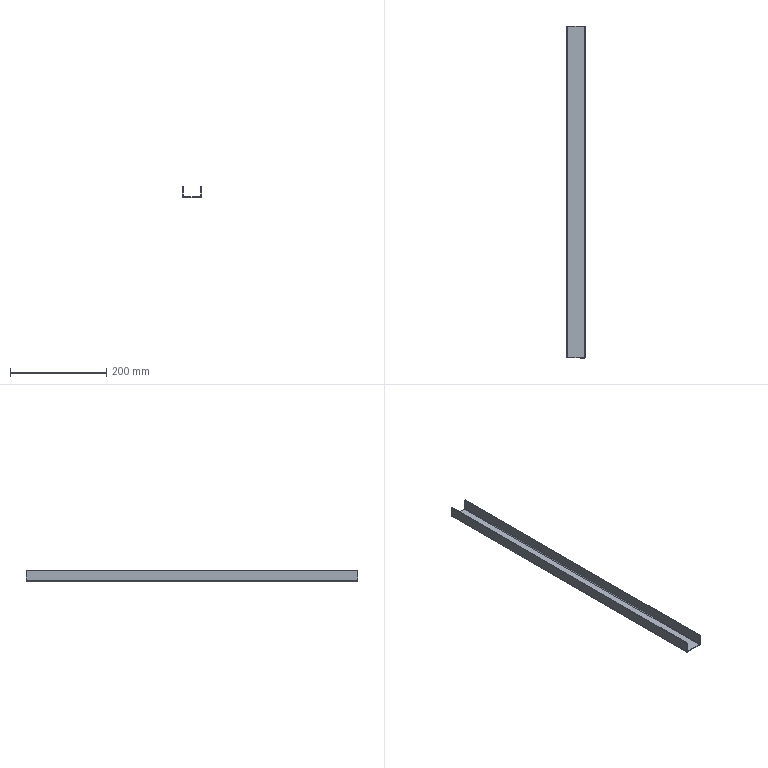Part | STEP file | Rear door reinforcing rib | 1 solid | 22 faces | box 40 x 691 x 23.5 mm | volume 85064 mm3 | plane 18 | cylinder 4 | commonest cylinder face diameters 3 x2 6 x2
STEP:
#1=CARTESIAN_POINT('',(0.,0.,0.));
#2=DIRECTION('',(0.,0.,1.));
#3=DIRECTION('',(1.,0.,0.));
#4=AXIS2_PLACEMENT_3D('',#1,#2,#3);
#5=CARTESIAN_POINT('',(-37.,0.,-1.5));
#6=VERTEX_POINT('',#5);
#7=CARTESIAN_POINT('',(-3.,0.,-1.5));
#8=VERTEX_POINT('',#7);
#9=CARTESIAN_POINT('',(0.,0.,-1.5));
#10=DIRECTION('',(1.,0.,0.));
#11=VECTOR('',#10,1.);
#12=LINE('',#9,#11);
#13=CARTESIAN_POINT('',(0.,0.,-1.5));
#14=DIRECTION('',(0.,0.,-1.));
#15=DIRECTION('',(-1.,0.,0.));
#16=AXIS2_PLACEMENT_3D('',#13,#14,#15);
#17=PLANE('',#16);
#18=CARTESIAN_POINT('',(0.,0.));
#19=DIRECTION('',(-1.,0.));
#20=VECTOR('',#19,1.);
#21=LINE('',#18,#20);
#22=(GEOMETRIC_REPRESENTATION_CONTEXT(2)PARAMETRIC_REPRESENTATION_CONTEXT()REPRESENTATION_CONTEXT('',''));
#23=DEFINITIONAL_REPRESENTATION('',(#21),#22);
#24=PCURVE('',#17,#23);
#25=CARTESIAN_POINT('',(0.,0.,-1.5));
#26=DIRECTION('',(0.,-1.,0.));
#27=DIRECTION('',(1.,0.,0.));
#28=AXIS2_PLACEMENT_3D('',#25,#26,#27);
#29=PLANE('',#28);
#30=CARTESIAN_POINT('',(0.,0.));
#31=DIRECTION('',(1.,0.));
#32=VECTOR('',#31,1.);
#33=LINE('',#30,#32);
#34=(GEOMETRIC_REPRESENTATION_CONTEXT(2)PARAMETRIC_REPRESENTATION_CONTEXT()REPRESENTATION_CONTEXT('',''));
#35=DEFINITIONAL_REPRESENTATION('',(#33),#34);
#36=PCURVE('',#29,#35);
#37=SURFACE_CURVE('',#12,(#24,#36),.PCURVE_S1.);
#38=EDGE_CURVE('',#6,#8,#37,.T.);
#39=ORIENTED_EDGE('',*,*,#38,.F.);
#40=CARTESIAN_POINT('',(-37.,691.,-1.5));
#41=VERTEX_POINT('',#40);
#42=CARTESIAN_POINT('',(-37.,0.,-1.5));
#43=DIRECTION('',(0.,1.,0.));
#44=VECTOR('',#43,1.);
#45=LINE('',#42,#44);
#46=CARTESIAN_POINT('',(37.,0.));
#47=DIRECTION('',(0.,1.));
#48=VECTOR('',#47,1.);
#49=LINE('',#46,#48);
#50=(GEOMETRIC_REPRESENTATION_CONTEXT(2)PARAMETRIC_REPRESENTATION_CONTEXT()REPRESENTATION_CONTEXT('',''));
#51=DEFINITIONAL_REPRESENTATION('',(#49),#50);
#52=PCURVE('',#17,#51);
#53=CARTESIAN_POINT('',(-37.,0.,1.5));
#54=DIRECTION('',(0.,-1.,0.));
#55=DIRECTION('',(-1.,0.,0.));
#56=AXIS2_PLACEMENT_3D('',#53,#54,#55);
#57=CYLINDRICAL_SURFACE('',#56,3.);
#58=CARTESIAN_POINT('',(1.571,0.));
#59=DIRECTION('',(0.,-1.));
#60=VECTOR('',#59,1.);
#61=LINE('',#58,#60);
#62=(GEOMETRIC_REPRESENTATION_CONTEXT(2)PARAMETRIC_REPRESENTATION_CONTEXT()REPRESENTATION_CONTEXT('',''));
#63=DEFINITIONAL_REPRESENTATION('',(#61),#62);
#64=PCURVE('',#57,#63);
#65=SURFACE_CURVE('',#45,(#52,#64),.PCURVE_S1.);
#66=EDGE_CURVE('',#6,#41,#65,.T.);
#67=ORIENTED_EDGE('',*,*,#66,.T.);
#68=CARTESIAN_POINT('',(-3.,691.,-1.5));
#69=VERTEX_POINT('',#68);
#70=CARTESIAN_POINT('',(0.,691.,-1.5));
#71=DIRECTION('',(-1.,0.,0.));
#72=VECTOR('',#71,1.);
#73=LINE('',#70,#72);
#74=CARTESIAN_POINT('',(0.,691.));
#75=DIRECTION('',(1.,0.));
#76=VECTOR('',#75,1.);
#77=LINE('',#74,#76);
#78=(GEOMETRIC_REPRESENTATION_CONTEXT(2)PARAMETRIC_REPRESENTATION_CONTEXT()REPRESENTATION_CONTEXT('',''));
#79=DEFINITIONAL_REPRESENTATION('',(#77),#78);
#80=PCURVE('',#17,#79);
#81=CARTESIAN_POINT('',(0.,691.,-1.5));
#82=DIRECTION('',(0.,1.,0.));
#83=DIRECTION('',(0.,0.,1.));
#84=AXIS2_PLACEMENT_3D('',#81,#82,#83);
#85=PLANE('',#84);
#86=CARTESIAN_POINT('',(0.,0.));
#87=DIRECTION('',(0.,-1.));
#88=VECTOR('',#87,1.);
#89=LINE('',#86,#88);
#90=(GEOMETRIC_REPRESENTATION_CONTEXT(2)PARAMETRIC_REPRESENTATION_CONTEXT()REPRESENTATION_CONTEXT('',''));
#91=DEFINITIONAL_REPRESENTATION('',(#89),#90);
#92=PCURVE('',#85,#91);
#93=SURFACE_CURVE('',#73,(#80,#92),.PCURVE_S1.);
#94=EDGE_CURVE('',#69,#41,#93,.T.);
#95=ORIENTED_EDGE('',*,*,#94,.F.);
#96=CARTESIAN_POINT('',(-3.,691.,-1.5));
#97=DIRECTION('',(0.,-1.,0.));
#98=VECTOR('',#97,1.);
#99=LINE('',#96,#98);
#100=CARTESIAN_POINT('',(3.,691.));
#101=DIRECTION('',(0.,-1.));
#102=VECTOR('',#101,1.);
#103=LINE('',#100,#102);
#104=(GEOMETRIC_REPRESENTATION_CONTEXT(2)PARAMETRIC_REPRESENTATION_CONTEXT()REPRESENTATION_CONTEXT('',''));
#105=DEFINITIONAL_REPRESENTATION('',(#103),#104);
#106=PCURVE('',#17,#105);
#107=CARTESIAN_POINT('',(-3.,691.,1.5));
#108=DIRECTION('',(0.,1.,0.));
#109=DIRECTION('',(1.,0.,0.));
#110=AXIS2_PLACEMENT_3D('',#107,#108,#109);
#111=CYLINDRICAL_SURFACE('',#110,3.);
#112=CARTESIAN_POINT('',(1.571,0.));
#113=DIRECTION('',(0.,-1.));
#114=VECTOR('',#113,1.);
#115=LINE('',#112,#114);
#116=(GEOMETRIC_REPRESENTATION_CONTEXT(2)PARAMETRIC_REPRESENTATION_CONTEXT()REPRESENTATION_CONTEXT('',''));
#117=DEFINITIONAL_REPRESENTATION('',(#115),#116);
#118=PCURVE('',#111,#117);
#119=SURFACE_CURVE('',#99,(#106,#118),.PCURVE_S1.);
#120=EDGE_CURVE('',#69,#8,#119,.T.);
#121=ORIENTED_EDGE('',*,*,#120,.T.);
#122=EDGE_LOOP('',(#39,#67,#95,#121));
#123=FACE_BOUND('',#122,.T.);
#124=ADVANCED_FACE('',(#123),#17,.T.);
#125=CARTESIAN_POINT('',(-37.,0.,0.));
#126=VERTEX_POINT('',#125);
#127=CARTESIAN_POINT('',(-37.,691.,0.));
#128=VERTEX_POINT('',#127);
#129=CARTESIAN_POINT('',(-37.,0.,0.));
#130=DIRECTION('',(0.,1.,0.));
#131=VECTOR('',#130,1.);
#132=LINE('',#129,#131);
#133=CARTESIAN_POINT('',(0.,0.,0.));
#134=DIRECTION('',(0.,0.,-1.));
#135=DIRECTION('',(-1.,0.,0.));
#136=AXIS2_PLACEMENT_3D('',#133,#134,#135);
#137=PLANE('',#136);
#138=CARTESIAN_POINT('',(37.,0.));
#139=DIRECTION('',(0.,1.));
#140=VECTOR('',#139,1.);
#141=LINE('',#138,#140);
#142=(GEOMETRIC_REPRESENTATION_CONTEXT(2)PARAMETRIC_REPRESENTATION_CONTEXT()REPRESENTATION_CONTEXT('',''));
#143=DEFINITIONAL_REPRESENTATION('',(#141),#142);
#144=PCURVE('',#137,#143);
#145=CARTESIAN_POINT('',(-37.,0.,1.5));
#146=DIRECTION('',(0.,-1.,0.));
#147=DIRECTION('',(-1.,0.,0.));
#148=AXIS2_PLACEMENT_3D('',#145,#146,#147);
#149=CYLINDRICAL_SURFACE('',#148,1.5);
#150=CARTESIAN_POINT('',(1.571,0.));
#151=DIRECTION('',(0.,-1.));
#152=VECTOR('',#151,1.);
#153=LINE('',#150,#152);
#154=(GEOMETRIC_REPRESENTATION_CONTEXT(2)PARAMETRIC_REPRESENTATION_CONTEXT()REPRESENTATION_CONTEXT('',''));
#155=DEFINITIONAL_REPRESENTATION('',(#153),#154);
#156=PCURVE('',#149,#155);
#157=SURFACE_CURVE('',#132,(#144,#156),.PCURVE_S1.);
#158=EDGE_CURVE('',#126,#128,#157,.T.);
#159=ORIENTED_EDGE('',*,*,#158,.F.);
#160=CARTESIAN_POINT('',(-3.,0.,0.));
#161=VERTEX_POINT('',#160);
#162=CARTESIAN_POINT('',(0.,0.,0.));
#163=DIRECTION('',(1.,0.,0.));
#164=VECTOR('',#163,1.);
#165=LINE('',#162,#164);
#166=CARTESIAN_POINT('',(0.,0.));
#167=DIRECTION('',(-1.,0.));
#168=VECTOR('',#167,1.);
#169=LINE('',#166,#168);
#170=(GEOMETRIC_REPRESENTATION_CONTEXT(2)PARAMETRIC_REPRESENTATION_CONTEXT()REPRESENTATION_CONTEXT('',''));
#171=DEFINITIONAL_REPRESENTATION('',(#169),#170);
#172=PCURVE('',#137,#171);
#173=CARTESIAN_POINT('',(0.,1.5));
#174=DIRECTION('',(1.,0.));
#175=VECTOR('',#174,1.);
#176=LINE('',#173,#175);
#177=(GEOMETRIC_REPRESENTATION_CONTEXT(2)PARAMETRIC_REPRESENTATION_CONTEXT()REPRESENTATION_CONTEXT('',''));
#178=DEFINITIONAL_REPRESENTATION('',(#176),#177);
#179=PCURVE('',#29,#178);
#180=SURFACE_CURVE('',#165,(#172,#179),.PCURVE_S1.);
#181=EDGE_CURVE('',#126,#161,#180,.T.);
#182=ORIENTED_EDGE('',*,*,#181,.T.);
#183=CARTESIAN_POINT('',(-3.,691.,0.));
#184=VERTEX_POINT('',#183);
#185=CARTESIAN_POINT('',(-3.,691.,0.));
#186=DIRECTION('',(0.,-1.,0.));
#187=VECTOR('',#186,1.);
#188=LINE('',#185,#187);
#189=CARTESIAN_POINT('',(3.,691.));
#190=DIRECTION('',(0.,-1.));
#191=VECTOR('',#190,1.);
#192=LINE('',#189,#191);
#193=(GEOMETRIC_REPRESENTATION_CONTEXT(2)PARAMETRIC_REPRESENTATION_CONTEXT()REPRESENTATION_CONTEXT('',''));
#194=DEFINITIONAL_REPRESENTATION('',(#192),#193);
#195=PCURVE('',#137,#194);
#196=CARTESIAN_POINT('',(-3.,691.,1.5));
#197=DIRECTION('',(0.,1.,0.));
#198=DIRECTION('',(1.,0.,0.));
#199=AXIS2_PLACEMENT_3D('',#196,#197,#198);
#200=CYLINDRICAL_SURFACE('',#199,1.5);
#201=CARTESIAN_POINT('',(1.571,0.));
#202=DIRECTION('',(0.,-1.));
#203=VECTOR('',#202,1.);
#204=LINE('',#201,#203);
#205=(GEOMETRIC_REPRESENTATION_CONTEXT(2)PARAMETRIC_REPRESENTATION_CONTEXT()REPRESENTATION_CONTEXT('',''));
#206=DEFINITIONAL_REPRESENTATION('',(#204),#205);
#207=PCURVE('',#200,#206);
#208=SURFACE_CURVE('',#188,(#195,#207),.PCURVE_S1.);
#209=EDGE_CURVE('',#184,#161,#208,.T.);
#210=ORIENTED_EDGE('',*,*,#209,.F.);
#211=CARTESIAN_POINT('',(0.,691.,0.));
#212=DIRECTION('',(-1.,0.,0.));
#213=VECTOR('',#212,1.);
#214=LINE('',#211,#213);
#215=CARTESIAN_POINT('',(0.,691.));
#216=DIRECTION('',(1.,0.));
#217=VECTOR('',#216,1.);
#218=LINE('',#215,#217);
#219=(GEOMETRIC_REPRESENTATION_CONTEXT(2)PARAMETRIC_REPRESENTATION_CONTEXT()REPRESENTATION_CONTEXT('',''));
#220=DEFINITIONAL_REPRESENTATION('',(#218),#219);
#221=PCURVE('',#137,#220);
#222=CARTESIAN_POINT('',(1.5,0.));
#223=DIRECTION('',(0.,-1.));
#224=VECTOR('',#223,1.);
#225=LINE('',#222,#224);
#226=(GEOMETRIC_REPRESENTATION_CONTEXT(2)PARAMETRIC_REPRESENTATION_CONTEXT()REPRESENTATION_CONTEXT('',''));
#227=DEFINITIONAL_REPRESENTATION('',(#225),#226);
#228=PCURVE('',#85,#227);
#229=SURFACE_CURVE('',#214,(#221,#228),.PCURVE_S1.);
#230=EDGE_CURVE('',#184,#128,#229,.T.);
#231=ORIENTED_EDGE('',*,*,#230,.T.);
#232=EDGE_LOOP('',(#159,#182,#210,#231));
#233=FACE_BOUND('',#232,.T.);
#234=ADVANCED_FACE('',(#233),#137,.F.);
#235=ORIENTED_EDGE('',*,*,#181,.F.);
#236=CARTESIAN_POINT('',(-37.,0.,0.));
#237=DIRECTION('',(0.,0.,-1.));
#238=VECTOR('',#237,1.);
#239=LINE('',#236,#238);
#240=CARTESIAN_POINT('',(-37.,1.5));
#241=DIRECTION('',(0.,-1.));
#242=VECTOR('',#241,1.);
#243=LINE('',#240,#242);
#244=(GEOMETRIC_REPRESENTATION_CONTEXT(2)PARAMETRIC_REPRESENTATION_CONTEXT()REPRESENTATION_CONTEXT('',''));
#245=DEFINITIONAL_REPRESENTATION('',(#243),#244);
#246=PCURVE('',#29,#245);
#247=CARTESIAN_POINT('',(-37.,0.,1.5));
#248=DIRECTION('',(0.,1.,0.));
#249=DIRECTION('',(0.,0.,1.));
#250=AXIS2_PLACEMENT_3D('',#247,#248,#249);
#251=PLANE('',#250);
#252=CARTESIAN_POINT('',(-1.5,0.));
#253=DIRECTION('',(-1.,0.));
#254=VECTOR('',#253,1.);
#255=LINE('',#252,#254);
#256=(GEOMETRIC_REPRESENTATION_CONTEXT(2)PARAMETRIC_REPRESENTATION_CONTEXT()REPRESENTATION_CONTEXT('',''));
#257=DEFINITIONAL_REPRESENTATION('',(#255),#256);
#258=PCURVE('',#251,#257);
#259=SURFACE_CURVE('',#239,(#246,#258),.PCURVE_S1.);
#260=EDGE_CURVE('',#126,#6,#259,.T.);
#261=ORIENTED_EDGE('',*,*,#260,.T.);
#262=ORIENTED_EDGE('',*,*,#38,.T.);
#263=CARTESIAN_POINT('',(-3.,0.,0.));
#264=DIRECTION('',(0.,0.,-1.));
#265=VECTOR('',#264,1.);
#266=LINE('',#263,#265);
#267=CARTESIAN_POINT('',(-3.,1.5));
#268=DIRECTION('',(0.,-1.));
#269=VECTOR('',#268,1.);
#270=LINE('',#267,#269);
#271=(GEOMETRIC_REPRESENTATION_CONTEXT(2)PARAMETRIC_REPRESENTATION_CONTEXT()REPRESENTATION_CONTEXT('',''));
#272=DEFINITIONAL_REPRESENTATION('',(#270),#271);
#273=PCURVE('',#29,#272);
#274=CARTESIAN_POINT('',(-3.,0.,1.5));
#275=DIRECTION('',(0.,-1.,0.));
#276=DIRECTION('',(1.,0.,0.));
#277=AXIS2_PLACEMENT_3D('',#274,#275,#276);
#278=PLANE('',#277);
#279=CARTESIAN_POINT('',(0.,-1.5));
#280=DIRECTION('',(0.,-1.));
#281=VECTOR('',#280,1.);
#282=LINE('',#279,#281);
#283=(GEOMETRIC_REPRESENTATION_CONTEXT(2)PARAMETRIC_REPRESENTATION_CONTEXT()REPRESENTATION_CONTEXT('',''));
#284=DEFINITIONAL_REPRESENTATION('',(#282),#283);
#285=PCURVE('',#278,#284);
#286=SURFACE_CURVE('',#266,(#273,#285),.PCURVE_S1.);
#287=EDGE_CURVE('',#161,#8,#286,.T.);
#288=ORIENTED_EDGE('',*,*,#287,.F.);
#289=EDGE_LOOP('',(#235,#261,#262,#288));
#290=FACE_BOUND('',#289,.T.);
#291=ADVANCED_FACE('',(#290),#29,.T.);
#292=CARTESIAN_POINT('',(-37.,691.,0.));
#293=DIRECTION('',(0.,0.,-1.));
#294=VECTOR('',#293,1.);
#295=LINE('',#292,#294);
#296=CARTESIAN_POINT('',(1.5,-37.));
#297=DIRECTION('',(-1.,0.));
#298=VECTOR('',#297,1.);
#299=LINE('',#296,#298);
#300=(GEOMETRIC_REPRESENTATION_CONTEXT(2)PARAMETRIC_REPRESENTATION_CONTEXT()REPRESENTATION_CONTEXT('',''));
#301=DEFINITIONAL_REPRESENTATION('',(#299),#300);
#302=PCURVE('',#85,#301);
#303=CARTESIAN_POINT('',(-37.,691.,1.5));
#304=DIRECTION('',(0.,1.,0.));
#305=DIRECTION('',(0.,0.,1.));
#306=AXIS2_PLACEMENT_3D('',#303,#304,#305);
#307=PLANE('',#306);
#308=CARTESIAN_POINT('',(-1.5,0.));
#309=DIRECTION('',(-1.,0.));
#310=VECTOR('',#309,1.);
#311=LINE('',#308,#310);
#312=(GEOMETRIC_REPRESENTATION_CONTEXT(2)PARAMETRIC_REPRESENTATION_CONTEXT()REPRESENTATION_CONTEXT('',''));
#313=DEFINITIONAL_REPRESENTATION('',(#311),#312);
#314=PCURVE('',#307,#313);
#315=SURFACE_CURVE('',#295,(#302,#314),.PCURVE_S1.);
#316=EDGE_CURVE('',#128,#41,#315,.T.);
#317=ORIENTED_EDGE('',*,*,#316,.F.);
#318=ORIENTED_EDGE('',*,*,#230,.F.);
#319=CARTESIAN_POINT('',(-3.,691.,0.));
#320=DIRECTION('',(0.,0.,-1.));
#321=VECTOR('',#320,1.);
#322=LINE('',#319,#321);
#323=CARTESIAN_POINT('',(1.5,-3.));
#324=DIRECTION('',(-1.,0.));
#325=VECTOR('',#324,1.);
#326=LINE('',#323,#325);
#327=(GEOMETRIC_REPRESENTATION_CONTEXT(2)PARAMETRIC_REPRESENTATION_CONTEXT()REPRESENTATION_CONTEXT('',''));
#328=DEFINITIONAL_REPRESENTATION('',(#326),#327);
#329=PCURVE('',#85,#328);
#330=CARTESIAN_POINT('',(-3.,691.,1.5));
#331=DIRECTION('',(0.,-1.,0.));
#332=DIRECTION('',(1.,0.,0.));
#333=AXIS2_PLACEMENT_3D('',#330,#331,#332);
#334=PLANE('',#333);
#335=CARTESIAN_POINT('',(0.,-1.5));
#336=DIRECTION('',(0.,-1.));
#337=VECTOR('',#336,1.);
#338=LINE('',#335,#337);
#339=(GEOMETRIC_REPRESENTATION_CONTEXT(2)PARAMETRIC_REPRESENTATION_CONTEXT()REPRESENTATION_CONTEXT('',''));
#340=DEFINITIONAL_REPRESENTATION('',(#338),#339);
#341=PCURVE('',#334,#340);
#342=SURFACE_CURVE('',#322,(#329,#341),.PCURVE_S1.);
#343=EDGE_CURVE('',#184,#69,#342,.T.);
#344=ORIENTED_EDGE('',*,*,#343,.T.);
#345=ORIENTED_EDGE('',*,*,#94,.T.);
#346=EDGE_LOOP('',(#317,#318,#344,#345));
#347=FACE_BOUND('',#346,.T.);
#348=ADVANCED_FACE('',(#347),#85,.T.);
#349=CARTESIAN_POINT('',(-1.5,0.,1.5));
#350=VERTEX_POINT('',#349);
#351=CARTESIAN_POINT('',(0.,0.,1.5));
#352=VERTEX_POINT('',#351);
#353=CARTESIAN_POINT('',(0.,0.,1.5));
#354=DIRECTION('',(1.,0.,0.));
#355=VECTOR('',#354,1.);
#356=LINE('',#353,#355);
#357=CARTESIAN_POINT('',(3.,0.));
#358=DIRECTION('',(1.,0.));
#359=VECTOR('',#358,1.);
#360=LINE('',#357,#359);
#361=(GEOMETRIC_REPRESENTATION_CONTEXT(2)PARAMETRIC_REPRESENTATION_CONTEXT()REPRESENTATION_CONTEXT('',''));
#362=DEFINITIONAL_REPRESENTATION('',(#360),#361);
#363=PCURVE('',#278,#362);
#364=CARTESIAN_POINT('',(0.,0.,0.));
#365=DIRECTION('',(0.,1.,0.));
#366=DIRECTION('',(-1.,0.,0.));
#367=AXIS2_PLACEMENT_3D('',#364,#365,#366);
#368=PLANE('',#367);
#369=CARTESIAN_POINT('',(0.,1.5));
#370=DIRECTION('',(-1.,0.));
#371=VECTOR('',#370,1.);
#372=LINE('',#369,#371);
#373=(GEOMETRIC_REPRESENTATION_CONTEXT(2)PARAMETRIC_REPRESENTATION_CONTEXT()REPRESENTATION_CONTEXT('',''));
#374=DEFINITIONAL_REPRESENTATION('',(#372),#373);
#375=PCURVE('',#368,#374);
#376=SURFACE_CURVE('',#356,(#363,#375),.PCURVE_S1.);
#377=EDGE_CURVE('',#350,#352,#376,.T.);
#378=ORIENTED_EDGE('',*,*,#377,.F.);
#379=CARTESIAN_POINT('',(-3.,0.,1.5));
#380=DIRECTION('',(0.,-1.,0.));
#381=DIRECTION('',(-1.,0.,0.));
#382=AXIS2_PLACEMENT_3D('',#379,#380,#381);
#383=CIRCLE('',#382,1.5);
#384=CARTESIAN_POINT('',(0.,0.));
#385=DIRECTION('',(-1.,0.));
#386=AXIS2_PLACEMENT_2D('',#384,#385);
#387=CIRCLE('',#386,1.5);
#388=(GEOMETRIC_REPRESENTATION_CONTEXT(2)PARAMETRIC_REPRESENTATION_CONTEXT()REPRESENTATION_CONTEXT('',''));
#389=DEFINITIONAL_REPRESENTATION('',(#387),#388);
#390=PCURVE('',#278,#389);
#391=CARTESIAN_POINT('',(3.142,-691.));
#392=DIRECTION('',(-1.,0.));
#393=VECTOR('',#392,1.);
#394=LINE('',#391,#393);
#395=(GEOMETRIC_REPRESENTATION_CONTEXT(2)PARAMETRIC_REPRESENTATION_CONTEXT()REPRESENTATION_CONTEXT('',''));
#396=DEFINITIONAL_REPRESENTATION('',(#394),#395);
#397=PCURVE('',#200,#396);
#398=SURFACE_CURVE('',#383,(#390,#397),.PCURVE_S1.);
#399=EDGE_CURVE('',#161,#350,#398,.T.);
#400=ORIENTED_EDGE('',*,*,#399,.F.);
#401=ORIENTED_EDGE('',*,*,#287,.T.);
#402=CARTESIAN_POINT('',(-3.,0.,1.5));
#403=DIRECTION('',(0.,-1.,0.));
#404=DIRECTION('',(-1.,0.,0.));
#405=AXIS2_PLACEMENT_3D('',#402,#403,#404);
#406=CIRCLE('',#405,3.);
#407=CARTESIAN_POINT('',(0.,0.));
#408=DIRECTION('',(-1.,0.));
#409=AXIS2_PLACEMENT_2D('',#407,#408);
#410=CIRCLE('',#409,3.);
#411=(GEOMETRIC_REPRESENTATION_CONTEXT(2)PARAMETRIC_REPRESENTATION_CONTEXT()REPRESENTATION_CONTEXT('',''));
#412=DEFINITIONAL_REPRESENTATION('',(#410),#411);
#413=PCURVE('',#278,#412);
#414=CARTESIAN_POINT('',(3.142,-691.));
#415=DIRECTION('',(-1.,0.));
#416=VECTOR('',#415,1.);
#417=LINE('',#414,#416);
#418=(GEOMETRIC_REPRESENTATION_CONTEXT(2)PARAMETRIC_REPRESENTATION_CONTEXT()REPRESENTATION_CONTEXT('',''));
#419=DEFINITIONAL_REPRESENTATION('',(#417),#418);
#420=PCURVE('',#111,#419);
#421=SURFACE_CURVE('',#406,(#413,#420),.PCURVE_S1.);
#422=EDGE_CURVE('',#8,#352,#421,.T.);
#423=ORIENTED_EDGE('',*,*,#422,.T.);
#424=EDGE_LOOP('',(#378,#400,#401,#423));
#425=FACE_BOUND('',#424,.T.);
#426=ADVANCED_FACE('',(#425),#278,.T.);
#427=CARTESIAN_POINT('',(-1.5,691.,1.5));
#428=VERTEX_POINT('',#427);
#429=CARTESIAN_POINT('',(-3.,691.,1.5));
#430=DIRECTION('',(0.,1.,0.));
#431=DIRECTION('',(-1.,0.,0.));
#432=AXIS2_PLACEMENT_3D('',#429,#430,#431);
#433=CIRCLE('',#432,1.5);
#434=CARTESIAN_POINT('',(-1.5,0.));
#435=CARTESIAN_POINT('',(-1.5,2.598));
#436=CARTESIAN_POINT('',(0.75,1.299));
#437=CARTESIAN_POINT('',(3.,0.));
#438=CARTESIAN_POINT('',(0.75,-1.299));
#439=CARTESIAN_POINT('',(-1.5,-2.598));
#440=CARTESIAN_POINT('',(-1.5,0.));
#441=(BOUNDED_CURVE()B_SPLINE_CURVE(2,(#434,#435,#436,#437,#438,#439,#440),.UNSPECIFIED.,.T.,.F.)B_SPLINE_CURVE_WITH_KNOTS((1,2,2,2,2,1),(-2.094,0.,2.094,4.189,6.283,8.378),.UNSPECIFIED.)CURVE()GEOMETRIC_REPRESENTATION_ITEM()RATIONAL_B_SPLINE_CURVE((1.,0.5,1.,0.5,1.,0.5,1.))REPRESENTATION_ITEM(''));
#442=(GEOMETRIC_REPRESENTATION_CONTEXT(2)PARAMETRIC_REPRESENTATION_CONTEXT()REPRESENTATION_CONTEXT('',''));
#443=DEFINITIONAL_REPRESENTATION('',(#441),#442);
#444=PCURVE('',#334,#443);
#445=CARTESIAN_POINT('',(-3.142,0.));
#446=DIRECTION('',(1.,0.));
#447=VECTOR('',#446,1.);
#448=LINE('',#445,#447);
#449=(GEOMETRIC_REPRESENTATION_CONTEXT(2)PARAMETRIC_REPRESENTATION_CONTEXT()REPRESENTATION_CONTEXT('',''));
#450=DEFINITIONAL_REPRESENTATION('',(#448),#449);
#451=PCURVE('',#200,#450);
#452=SURFACE_CURVE('',#433,(#444,#451),.PCURVE_S1.);
#453=EDGE_CURVE('',#428,#184,#452,.T.);
#454=ORIENTED_EDGE('',*,*,#453,.F.);
#455=CARTESIAN_POINT('',(0.,691.,1.5));
#456=VERTEX_POINT('',#455);
#457=CARTESIAN_POINT('',(-1.5,691.,1.5));
#458=DIRECTION('',(1.,0.,0.));
#459=VECTOR('',#458,1.);
#460=LINE('',#457,#459);
#461=CARTESIAN_POINT('',(1.5,0.));
#462=DIRECTION('',(1.,0.));
#463=VECTOR('',#462,1.);
#464=LINE('',#461,#463);
#465=(GEOMETRIC_REPRESENTATION_CONTEXT(2)PARAMETRIC_REPRESENTATION_CONTEXT()REPRESENTATION_CONTEXT('',''));
#466=DEFINITIONAL_REPRESENTATION('',(#464),#465);
#467=PCURVE('',#334,#466);
#468=CARTESIAN_POINT('',(0.,691.,22.));
#469=DIRECTION('',(0.,-1.,0.));
#470=DIRECTION('',(1.,0.,0.));
#471=AXIS2_PLACEMENT_3D('',#468,#469,#470);
#472=PLANE('',#471);
#473=CARTESIAN_POINT('',(-1.5,-20.5));
#474=DIRECTION('',(1.,0.));
#475=VECTOR('',#474,1.);
#476=LINE('',#473,#475);
#477=(GEOMETRIC_REPRESENTATION_CONTEXT(2)PARAMETRIC_REPRESENTATION_CONTEXT()REPRESENTATION_CONTEXT('',''));
#478=DEFINITIONAL_REPRESENTATION('',(#476),#477);
#479=PCURVE('',#472,#478);
#480=SURFACE_CURVE('',#460,(#467,#479),.PCURVE_S1.);
#481=EDGE_CURVE('',#428,#456,#480,.T.);
#482=ORIENTED_EDGE('',*,*,#481,.T.);
#483=CARTESIAN_POINT('',(-3.,691.,1.5));
#484=DIRECTION('',(0.,1.,0.));
#485=DIRECTION('',(-1.,0.,0.));
#486=AXIS2_PLACEMENT_3D('',#483,#484,#485);
#487=CIRCLE('',#486,3.);
#488=CARTESIAN_POINT('',(-3.,0.));
#489=CARTESIAN_POINT('',(-3.,5.196));
#490=CARTESIAN_POINT('',(1.5,2.598));
#491=CARTESIAN_POINT('',(6.,0.));
#492=CARTESIAN_POINT('',(1.5,-2.598));
#493=CARTESIAN_POINT('',(-3.,-5.196));
#494=CARTESIAN_POINT('',(-3.,0.));
#495=(BOUNDED_CURVE()B_SPLINE_CURVE(2,(#488,#489,#490,#491,#492,#493,#494),.UNSPECIFIED.,.T.,.F.)B_SPLINE_CURVE_WITH_KNOTS((1,2,2,2,2,1),(-2.094,0.,2.094,4.189,6.283,8.378),.UNSPECIFIED.)CURVE()GEOMETRIC_REPRESENTATION_ITEM()RATIONAL_B_SPLINE_CURVE((1.,0.5,1.,0.5,1.,0.5,1.))REPRESENTATION_ITEM(''));
#496=(GEOMETRIC_REPRESENTATION_CONTEXT(2)PARAMETRIC_REPRESENTATION_CONTEXT()REPRESENTATION_CONTEXT('',''));
#497=DEFINITIONAL_REPRESENTATION('',(#495),#496);
#498=PCURVE('',#334,#497);
#499=CARTESIAN_POINT('',(-3.142,0.));
#500=DIRECTION('',(1.,0.));
#501=VECTOR('',#500,1.);
#502=LINE('',#499,#501);
#503=(GEOMETRIC_REPRESENTATION_CONTEXT(2)PARAMETRIC_REPRESENTATION_CONTEXT()REPRESENTATION_CONTEXT('',''));
#504=DEFINITIONAL_REPRESENTATION('',(#502),#503);
#505=PCURVE('',#111,#504);
#506=SURFACE_CURVE('',#487,(#498,#505),.PCURVE_S1.);
#507=EDGE_CURVE('',#456,#69,#506,.T.);
#508=ORIENTED_EDGE('',*,*,#507,.T.);
#509=ORIENTED_EDGE('',*,*,#343,.F.);
#510=EDGE_LOOP('',(#454,#482,#508,#509));
#511=FACE_BOUND('',#510,.T.);
#512=ADVANCED_FACE('',(#511),#334,.F.);
#513=ORIENTED_EDGE('',*,*,#120,.F.);
#514=ORIENTED_EDGE('',*,*,#507,.F.);
#515=CARTESIAN_POINT('',(0.,0.,1.5));
#516=DIRECTION('',(0.,-1.,0.));
#517=VECTOR('',#516,1.);
#518=LINE('',#515,#517);
#519=CARTESIAN_POINT('',(0.,-691.));
#520=DIRECTION('',(0.,-1.));
#521=VECTOR('',#520,1.);
#522=LINE('',#519,#521);
#523=(GEOMETRIC_REPRESENTATION_CONTEXT(2)PARAMETRIC_REPRESENTATION_CONTEXT()REPRESENTATION_CONTEXT('',''));
#524=DEFINITIONAL_REPRESENTATION('',(#522),#523);
#525=PCURVE('',#111,#524);
#526=CARTESIAN_POINT('',(0.,0.,0.));
#527=DIRECTION('',(-1.,0.,0.));
#528=DIRECTION('',(0.,0.,1.));
#529=AXIS2_PLACEMENT_3D('',#526,#527,#528);
#530=PLANE('',#529);
#531=CARTESIAN_POINT('',(1.5,0.));
#532=DIRECTION('',(0.,-1.));
#533=VECTOR('',#532,1.);
#534=LINE('',#531,#533);
#535=(GEOMETRIC_REPRESENTATION_CONTEXT(2)PARAMETRIC_REPRESENTATION_CONTEXT()REPRESENTATION_CONTEXT('',''));
#536=DEFINITIONAL_REPRESENTATION('',(#534),#535);
#537=PCURVE('',#530,#536);
#538=SURFACE_CURVE('',#518,(#525,#537),.PCURVE_S1.);
#539=EDGE_CURVE('',#456,#352,#538,.T.);
#540=ORIENTED_EDGE('',*,*,#539,.T.);
#541=ORIENTED_EDGE('',*,*,#422,.F.);
#542=EDGE_LOOP('',(#513,#514,#540,#541));
#543=FACE_BOUND('',#542,.T.);
#544=ADVANCED_FACE('',(#543),#111,.T.);
#545=ORIENTED_EDGE('',*,*,#453,.F.);
#546=CARTESIAN_POINT('',(-1.5,0.,1.5));
#547=DIRECTION('',(0.,1.,0.));
#548=VECTOR('',#547,1.);
#549=LINE('',#546,#548);
#550=CARTESIAN_POINT('',(0.,-691.));
#551=DIRECTION('',(0.,1.));
#552=VECTOR('',#551,1.);
#553=LINE('',#550,#552);
#554=(GEOMETRIC_REPRESENTATION_CONTEXT(2)PARAMETRIC_REPRESENTATION_CONTEXT()REPRESENTATION_CONTEXT('',''));
#555=DEFINITIONAL_REPRESENTATION('',(#553),#554);
#556=PCURVE('',#200,#555);
#557=CARTESIAN_POINT('',(-1.5,0.,0.));
#558=DIRECTION('',(-1.,0.,0.));
#559=DIRECTION('',(0.,0.,1.));
#560=AXIS2_PLACEMENT_3D('',#557,#558,#559);
#561=PLANE('',#560);
#562=CARTESIAN_POINT('',(1.5,0.));
#563=DIRECTION('',(0.,1.));
#564=VECTOR('',#563,1.);
#565=LINE('',#562,#564);
#566=(GEOMETRIC_REPRESENTATION_CONTEXT(2)PARAMETRIC_REPRESENTATION_CONTEXT()REPRESENTATION_CONTEXT('',''));
#567=DEFINITIONAL_REPRESENTATION('',(#565),#566);
#568=PCURVE('',#561,#567);
#569=SURFACE_CURVE('',#549,(#556,#568),.PCURVE_S1.);
#570=EDGE_CURVE('',#350,#428,#569,.T.);
#571=ORIENTED_EDGE('',*,*,#570,.F.);
#572=ORIENTED_EDGE('',*,*,#399,.F.);
#573=ORIENTED_EDGE('',*,*,#209,.F.);
#574=EDGE_LOOP('',(#545,#571,#572,#573));
#575=FACE_BOUND('',#574,.F.);
#576=ADVANCED_FACE('',(#575),#200,.F.);
#577=ORIENTED_EDGE('',*,*,#377,.T.);
#578=CARTESIAN_POINT('',(0.,0.,22.));
#579=VERTEX_POINT('',#578);
#580=CARTESIAN_POINT('',(0.,0.,0.));
#581=DIRECTION('',(0.,0.,-1.));
#582=VECTOR('',#581,1.);
#583=LINE('',#580,#582);
#584=CARTESIAN_POINT('',(0.,0.));
#585=DIRECTION('',(0.,-1.));
#586=VECTOR('',#585,1.);
#587=LINE('',#584,#586);
#588=(GEOMETRIC_REPRESENTATION_CONTEXT(2)PARAMETRIC_REPRESENTATION_CONTEXT()REPRESENTATION_CONTEXT('',''));
#589=DEFINITIONAL_REPRESENTATION('',(#587),#588);
#590=PCURVE('',#368,#589);
#591=CARTESIAN_POINT('',(0.,0.));
#592=DIRECTION('',(-1.,0.));
#593=VECTOR('',#592,1.);
#594=LINE('',#591,#593);
#595=(GEOMETRIC_REPRESENTATION_CONTEXT(2)PARAMETRIC_REPRESENTATION_CONTEXT()REPRESENTATION_CONTEXT('',''));
#596=DEFINITIONAL_REPRESENTATION('',(#594),#595);
#597=PCURVE('',#530,#596);
#598=SURFACE_CURVE('',#583,(#590,#597),.PCURVE_S1.);
#599=EDGE_CURVE('',#579,#352,#598,.T.);
#600=ORIENTED_EDGE('',*,*,#599,.F.);
#601=CARTESIAN_POINT('',(-1.5,0.,22.));
#602=VERTEX_POINT('',#601);
#603=CARTESIAN_POINT('',(0.,0.,22.));
#604=DIRECTION('',(-1.,0.,0.));
#605=VECTOR('',#604,1.);
#606=LINE('',#603,#605);
#607=CARTESIAN_POINT('',(0.,22.));
#608=DIRECTION('',(1.,0.));
#609=VECTOR('',#608,1.);
#610=LINE('',#607,#609);
#611=(GEOMETRIC_REPRESENTATION_CONTEXT(2)PARAMETRIC_REPRESENTATION_CONTEXT()REPRESENTATION_CONTEXT('',''));
#612=DEFINITIONAL_REPRESENTATION('',(#610),#611);
#613=PCURVE('',#368,#612);
#614=CARTESIAN_POINT('',(0.,0.,22.));
#615=DIRECTION('',(0.,0.,-1.));
#616=DIRECTION('',(-1.,0.,0.));
#617=AXIS2_PLACEMENT_3D('',#614,#615,#616);
#618=PLANE('',#617);
#619=CARTESIAN_POINT('',(0.,0.));
#620=DIRECTION('',(1.,0.));
#621=VECTOR('',#620,1.);
#622=LINE('',#619,#621);
#623=(GEOMETRIC_REPRESENTATION_CONTEXT(2)PARAMETRIC_REPRESENTATION_CONTEXT()REPRESENTATION_CONTEXT('',''));
#624=DEFINITIONAL_REPRESENTATION('',(#622),#623);
#625=PCURVE('',#618,#624);
#626=SURFACE_CURVE('',#606,(#613,#625),.PCURVE_S1.);
#627=EDGE_CURVE('',#579,#602,#626,.T.);
#628=ORIENTED_EDGE('',*,*,#627,.T.);
#629=CARTESIAN_POINT('',(-1.5,0.,0.));
#630=DIRECTION('',(0.,0.,-1.));
#631=VECTOR('',#630,1.);
#632=LINE('',#629,#631);
#633=CARTESIAN_POINT('',(1.5,0.));
#634=DIRECTION('',(0.,-1.));
#635=VECTOR('',#634,1.);
#636=LINE('',#633,#635);
#637=(GEOMETRIC_REPRESENTATION_CONTEXT(2)PARAMETRIC_REPRESENTATION_CONTEXT()REPRESENTATION_CONTEXT('',''));
#638=DEFINITIONAL_REPRESENTATION('',(#636),#637);
#639=PCURVE('',#368,#638);
#640=CARTESIAN_POINT('',(0.,0.));
#641=DIRECTION('',(-1.,0.));
#642=VECTOR('',#641,1.);
#643=LINE('',#640,#642);
#644=(GEOMETRIC_REPRESENTATION_CONTEXT(2)PARAMETRIC_REPRESENTATION_CONTEXT()REPRESENTATION_CONTEXT('',''));
#645=DEFINITIONAL_REPRESENTATION('',(#643),#644);
#646=PCURVE('',#561,#645);
#647=SURFACE_CURVE('',#632,(#639,#646),.PCURVE_S1.);
#648=EDGE_CURVE('',#602,#350,#647,.T.);
#649=ORIENTED_EDGE('',*,*,#648,.T.);
#650=EDGE_LOOP('',(#577,#600,#628,#649));
#651=FACE_BOUND('',#650,.T.);
#652=ADVANCED_FACE('',(#651),#368,.F.);
#653=ORIENTED_EDGE('',*,*,#481,.F.);
#654=CARTESIAN_POINT('',(-1.5,691.,22.));
#655=VERTEX_POINT('',#654);
#656=CARTESIAN_POINT('',(-1.5,691.,22.));
#657=DIRECTION('',(0.,0.,1.));
#658=VECTOR('',#657,1.);
#659=LINE('',#656,#658);
#660=CARTESIAN_POINT('',(-1.5,0.));
#661=DIRECTION('',(0.,1.));
#662=VECTOR('',#661,1.);
#663=LINE('',#660,#662);
#664=(GEOMETRIC_REPRESENTATION_CONTEXT(2)PARAMETRIC_REPRESENTATION_CONTEXT()REPRESENTATION_CONTEXT('',''));
#665=DEFINITIONAL_REPRESENTATION('',(#663),#664);
#666=PCURVE('',#472,#665);
#667=CARTESIAN_POINT('',(22.,691.));
#668=DIRECTION('',(1.,0.));
#669=VECTOR('',#668,1.);
#670=LINE('',#667,#669);
#671=(GEOMETRIC_REPRESENTATION_CONTEXT(2)PARAMETRIC_REPRESENTATION_CONTEXT()REPRESENTATION_CONTEXT('',''));
#672=DEFINITIONAL_REPRESENTATION('',(#670),#671);
#673=PCURVE('',#561,#672);
#674=SURFACE_CURVE('',#659,(#666,#673),.PCURVE_S1.);
#675=EDGE_CURVE('',#428,#655,#674,.T.);
#676=ORIENTED_EDGE('',*,*,#675,.T.);
#677=CARTESIAN_POINT('',(0.,691.,22.));
#678=VERTEX_POINT('',#677);
#679=CARTESIAN_POINT('',(0.,691.,22.));
#680=DIRECTION('',(-1.,0.,0.));
#681=VECTOR('',#680,1.);
#682=LINE('',#679,#681);
#683=CARTESIAN_POINT('',(0.,0.));
#684=DIRECTION('',(-1.,0.));
#685=VECTOR('',#684,1.);
#686=LINE('',#683,#685);
#687=(GEOMETRIC_REPRESENTATION_CONTEXT(2)PARAMETRIC_REPRESENTATION_CONTEXT()REPRESENTATION_CONTEXT('',''));
#688=DEFINITIONAL_REPRESENTATION('',(#686),#687);
#689=PCURVE('',#472,#688);
#690=CARTESIAN_POINT('',(0.,691.));
#691=DIRECTION('',(1.,0.));
#692=VECTOR('',#691,1.);
#693=LINE('',#690,#692);
#694=(GEOMETRIC_REPRESENTATION_CONTEXT(2)PARAMETRIC_REPRESENTATION_CONTEXT()REPRESENTATION_CONTEXT('',''));
#695=DEFINITIONAL_REPRESENTATION('',(#693),#694);
#696=PCURVE('',#618,#695);
#697=SURFACE_CURVE('',#682,(#689,#696),.PCURVE_S1.);
#698=EDGE_CURVE('',#678,#655,#697,.T.);
#699=ORIENTED_EDGE('',*,*,#698,.F.);
#700=CARTESIAN_POINT('',(0.,691.,0.));
#701=DIRECTION('',(0.,0.,1.));
#702=VECTOR('',#701,1.);
#703=LINE('',#700,#702);
#704=CARTESIAN_POINT('',(0.,-22.));
#705=DIRECTION('',(0.,1.));
#706=VECTOR('',#705,1.);
#707=LINE('',#704,#706);
#708=(GEOMETRIC_REPRESENTATION_CONTEXT(2)PARAMETRIC_REPRESENTATION_CONTEXT()REPRESENTATION_CONTEXT('',''));
#709=DEFINITIONAL_REPRESENTATION('',(#707),#708);
#710=PCURVE('',#472,#709);
#711=CARTESIAN_POINT('',(0.,691.));
#712=DIRECTION('',(1.,0.));
#713=VECTOR('',#712,1.);
#714=LINE('',#711,#713);
#715=(GEOMETRIC_REPRESENTATION_CONTEXT(2)PARAMETRIC_REPRESENTATION_CONTEXT()REPRESENTATION_CONTEXT('',''));
#716=DEFINITIONAL_REPRESENTATION('',(#714),#715);
#717=PCURVE('',#530,#716);
#718=SURFACE_CURVE('',#703,(#710,#717),.PCURVE_S1.);
#719=EDGE_CURVE('',#456,#678,#718,.T.);
#720=ORIENTED_EDGE('',*,*,#719,.F.);
#721=EDGE_LOOP('',(#653,#676,#699,#720));
#722=FACE_BOUND('',#721,.T.);
#723=ADVANCED_FACE('',(#722),#472,.F.);
#724=ORIENTED_EDGE('',*,*,#539,.F.);
#725=ORIENTED_EDGE('',*,*,#719,.T.);
#726=CARTESIAN_POINT('',(0.,0.,22.));
#727=DIRECTION('',(0.,-1.,0.));
#728=VECTOR('',#727,1.);
#729=LINE('',#726,#728);
#730=CARTESIAN_POINT('',(22.,0.));
#731=DIRECTION('',(0.,-1.));
#732=VECTOR('',#731,1.);
#733=LINE('',#730,#732);
#734=(GEOMETRIC_REPRESENTATION_CONTEXT(2)PARAMETRIC_REPRESENTATION_CONTEXT()REPRESENTATION_CONTEXT('',''));
#735=DEFINITIONAL_REPRESENTATION('',(#733),#734);
#736=PCURVE('',#530,#735);
#737=CARTESIAN_POINT('',(0.,0.));
#738=DIRECTION('',(0.,-1.));
#739=VECTOR('',#738,1.);
#740=LINE('',#737,#739);
#741=(GEOMETRIC_REPRESENTATION_CONTEXT(2)PARAMETRIC_REPRESENTATION_CONTEXT()REPRESENTATION_CONTEXT('',''));
#742=DEFINITIONAL_REPRESENTATION('',(#740),#741);
#743=PCURVE('',#618,#742);
#744=SURFACE_CURVE('',#729,(#736,#743),.PCURVE_S1.);
#745=EDGE_CURVE('',#678,#579,#744,.T.);
#746=ORIENTED_EDGE('',*,*,#745,.T.);
#747=ORIENTED_EDGE('',*,*,#599,.T.);
#748=EDGE_LOOP('',(#724,#725,#746,#747));
#749=FACE_BOUND('',#748,.T.);
#750=ADVANCED_FACE('',(#749),#530,.F.);
#751=ORIENTED_EDGE('',*,*,#675,.F.);
#752=ORIENTED_EDGE('',*,*,#570,.F.);
#753=ORIENTED_EDGE('',*,*,#648,.F.);
#754=CARTESIAN_POINT('',(-1.5,0.,22.));
#755=DIRECTION('',(0.,-1.,0.));
#756=VECTOR('',#755,1.);
#757=LINE('',#754,#756);
#758=CARTESIAN_POINT('',(22.,0.));
#759=DIRECTION('',(0.,-1.));
#760=VECTOR('',#759,1.);
#761=LINE('',#758,#760);
#762=(GEOMETRIC_REPRESENTATION_CONTEXT(2)PARAMETRIC_REPRESENTATION_CONTEXT()REPRESENTATION_CONTEXT('',''));
#763=DEFINITIONAL_REPRESENTATION('',(#761),#762);
#764=PCURVE('',#561,#763);
#765=CARTESIAN_POINT('',(1.5,0.));
#766=DIRECTION('',(0.,-1.));
#767=VECTOR('',#766,1.);
#768=LINE('',#765,#767);
#769=(GEOMETRIC_REPRESENTATION_CONTEXT(2)PARAMETRIC_REPRESENTATION_CONTEXT()REPRESENTATION_CONTEXT('',''));
#770=DEFINITIONAL_REPRESENTATION('',(#768),#769);
#771=PCURVE('',#618,#770);
#772=SURFACE_CURVE('',#757,(#764,#771),.PCURVE_S1.);
#773=EDGE_CURVE('',#655,#602,#772,.T.);
#774=ORIENTED_EDGE('',*,*,#773,.F.);
#775=EDGE_LOOP('',(#751,#752,#753,#774));
#776=FACE_BOUND('',#775,.T.);
#777=ADVANCED_FACE('',(#776),#561,.T.);
#778=ORIENTED_EDGE('',*,*,#773,.T.);
#779=ORIENTED_EDGE('',*,*,#627,.F.);
#780=ORIENTED_EDGE('',*,*,#745,.F.);
#781=ORIENTED_EDGE('',*,*,#698,.T.);
#782=EDGE_LOOP('',(#778,#779,#780,#781));
#783=FACE_BOUND('',#782,.T.);
#784=ADVANCED_FACE('',(#783),#618,.F.);
#785=CARTESIAN_POINT('',(-38.5,691.,1.5));
#786=VERTEX_POINT('',#785);
#787=CARTESIAN_POINT('',(-40.,691.,1.5));
#788=VERTEX_POINT('',#787);
#789=CARTESIAN_POINT('',(-40.,691.,1.5));
#790=DIRECTION('',(-1.,0.,0.));
#791=VECTOR('',#790,1.);
#792=LINE('',#789,#791);
#793=CARTESIAN_POINT('',(0.,-3.));
#794=DIRECTION('',(0.,-1.));
#795=VECTOR('',#794,1.);
#796=LINE('',#793,#795);
#797=(GEOMETRIC_REPRESENTATION_CONTEXT(2)PARAMETRIC_REPRESENTATION_CONTEXT()REPRESENTATION_CONTEXT('',''));
#798=DEFINITIONAL_REPRESENTATION('',(#796),#797);
#799=PCURVE('',#307,#798);
#800=CARTESIAN_POINT('',(-40.,691.,0.));
#801=DIRECTION('',(0.,-1.,0.));
#802=DIRECTION('',(1.,0.,0.));
#803=AXIS2_PLACEMENT_3D('',#800,#801,#802);
#804=PLANE('',#803);
#805=CARTESIAN_POINT('',(0.,1.5));
#806=DIRECTION('',(-1.,0.));
#807=VECTOR('',#806,1.);
#808=LINE('',#805,#807);
#809=(GEOMETRIC_REPRESENTATION_CONTEXT(2)PARAMETRIC_REPRESENTATION_CONTEXT()REPRESENTATION_CONTEXT('',''));
#810=DEFINITIONAL_REPRESENTATION('',(#808),#809);
#811=PCURVE('',#804,#810);
#812=SURFACE_CURVE('',#792,(#799,#811),.PCURVE_S1.);
#813=EDGE_CURVE('',#786,#788,#812,.T.);
#814=ORIENTED_EDGE('',*,*,#813,.F.);
#815=CARTESIAN_POINT('',(-37.,691.,1.5));
#816=DIRECTION('',(0.,1.,0.));
#817=DIRECTION('',(0.,0.,-1.));
#818=AXIS2_PLACEMENT_3D('',#815,#816,#817);
#819=CIRCLE('',#818,1.5);
#820=CARTESIAN_POINT('',(0.,0.));
#821=DIRECTION('',(-1.,0.));
#822=AXIS2_PLACEMENT_2D('',#820,#821);
#823=CIRCLE('',#822,1.5);
#824=(GEOMETRIC_REPRESENTATION_CONTEXT(2)PARAMETRIC_REPRESENTATION_CONTEXT()REPRESENTATION_CONTEXT('',''));
#825=DEFINITIONAL_REPRESENTATION('',(#823),#824);
#826=PCURVE('',#307,#825);
#827=CARTESIAN_POINT('',(1.571,-691.));
#828=DIRECTION('',(-1.,0.));
#829=VECTOR('',#828,1.);
#830=LINE('',#827,#829);
#831=(GEOMETRIC_REPRESENTATION_CONTEXT(2)PARAMETRIC_REPRESENTATION_CONTEXT()REPRESENTATION_CONTEXT('',''));
#832=DEFINITIONAL_REPRESENTATION('',(#830),#831);
#833=PCURVE('',#149,#832);
#834=SURFACE_CURVE('',#819,(#826,#833),.PCURVE_S1.);
#835=EDGE_CURVE('',#128,#786,#834,.T.);
#836=ORIENTED_EDGE('',*,*,#835,.F.);
#837=ORIENTED_EDGE('',*,*,#316,.T.);
#838=CARTESIAN_POINT('',(-37.,691.,1.5));
#839=DIRECTION('',(0.,1.,0.));
#840=DIRECTION('',(0.,0.,-1.));
#841=AXIS2_PLACEMENT_3D('',#838,#839,#840);
#842=CIRCLE('',#841,3.);
#843=CARTESIAN_POINT('',(0.,0.));
#844=DIRECTION('',(-1.,0.));
#845=AXIS2_PLACEMENT_2D('',#843,#844);
#846=CIRCLE('',#845,3.);
#847=(GEOMETRIC_REPRESENTATION_CONTEXT(2)PARAMETRIC_REPRESENTATION_CONTEXT()REPRESENTATION_CONTEXT('',''));
#848=DEFINITIONAL_REPRESENTATION('',(#846),#847);
#849=PCURVE('',#307,#848);
#850=CARTESIAN_POINT('',(1.571,-691.));
#851=DIRECTION('',(-1.,0.));
#852=VECTOR('',#851,1.);
#853=LINE('',#850,#852);
#854=(GEOMETRIC_REPRESENTATION_CONTEXT(2)PARAMETRIC_REPRESENTATION_CONTEXT()REPRESENTATION_CONTEXT('',''));
#855=DEFINITIONAL_REPRESENTATION('',(#853),#854);
#856=PCURVE('',#57,#855);
#857=SURFACE_CURVE('',#842,(#849,#856),.PCURVE_S1.);
#858=EDGE_CURVE('',#41,#788,#857,.T.);
#859=ORIENTED_EDGE('',*,*,#858,.T.);
#860=EDGE_LOOP('',(#814,#836,#837,#859));
#861=FACE_BOUND('',#860,.T.);
#862=ADVANCED_FACE('',(#861),#307,.T.);
#863=CARTESIAN_POINT('',(-38.5,0.,1.5));
#864=VERTEX_POINT('',#863);
#865=CARTESIAN_POINT('',(-37.,0.,1.5));
#866=DIRECTION('',(0.,-1.,0.));
#867=DIRECTION('',(0.,0.,-1.));
#868=AXIS2_PLACEMENT_3D('',#865,#866,#867);
#869=CIRCLE('',#868,1.5);
#870=CARTESIAN_POINT('',(-1.5,0.));
#871=CARTESIAN_POINT('',(-1.5,2.598));
#872=CARTESIAN_POINT('',(0.75,1.299));
#873=CARTESIAN_POINT('',(3.,0.));
#874=CARTESIAN_POINT('',(0.75,-1.299));
#875=CARTESIAN_POINT('',(-1.5,-2.598));
#876=CARTESIAN_POINT('',(-1.5,0.));
#877=(BOUNDED_CURVE()B_SPLINE_CURVE(2,(#870,#871,#872,#873,#874,#875,#876),.UNSPECIFIED.,.T.,.F.)B_SPLINE_CURVE_WITH_KNOTS((1,2,2,2,2,1),(-2.094,0.,2.094,4.189,6.283,8.378),.UNSPECIFIED.)CURVE()GEOMETRIC_REPRESENTATION_ITEM()RATIONAL_B_SPLINE_CURVE((1.,0.5,1.,0.5,1.,0.5,1.))REPRESENTATION_ITEM(''));
#878=(GEOMETRIC_REPRESENTATION_CONTEXT(2)PARAMETRIC_REPRESENTATION_CONTEXT()REPRESENTATION_CONTEXT('',''));
#879=DEFINITIONAL_REPRESENTATION('',(#877),#878);
#880=PCURVE('',#251,#879);
#881=CARTESIAN_POINT('',(-4.712,0.));
#882=DIRECTION('',(1.,0.));
#883=VECTOR('',#882,1.);
#884=LINE('',#881,#883);
#885=(GEOMETRIC_REPRESENTATION_CONTEXT(2)PARAMETRIC_REPRESENTATION_CONTEXT()REPRESENTATION_CONTEXT('',''));
#886=DEFINITIONAL_REPRESENTATION('',(#884),#885);
#887=PCURVE('',#149,#886);
#888=SURFACE_CURVE('',#869,(#880,#887),.PCURVE_S1.);
#889=EDGE_CURVE('',#864,#126,#888,.T.);
#890=ORIENTED_EDGE('',*,*,#889,.F.);
#891=CARTESIAN_POINT('',(-40.,0.,1.5));
#892=VERTEX_POINT('',#891);
#893=CARTESIAN_POINT('',(-38.5,0.,1.5));
#894=DIRECTION('',(-1.,0.,0.));
#895=VECTOR('',#894,1.);
#896=LINE('',#893,#895);
#897=CARTESIAN_POINT('',(0.,-1.5));
#898=DIRECTION('',(0.,-1.));
#899=VECTOR('',#898,1.);
#900=LINE('',#897,#899);
#901=(GEOMETRIC_REPRESENTATION_CONTEXT(2)PARAMETRIC_REPRESENTATION_CONTEXT()REPRESENTATION_CONTEXT('',''));
#902=DEFINITIONAL_REPRESENTATION('',(#900),#901);
#903=PCURVE('',#251,#902);
#904=CARTESIAN_POINT('',(-40.,0.,22.));
#905=DIRECTION('',(0.,1.,0.));
#906=DIRECTION('',(0.,0.,1.));
#907=AXIS2_PLACEMENT_3D('',#904,#905,#906);
#908=PLANE('',#907);
#909=CARTESIAN_POINT('',(-20.5,1.5));
#910=DIRECTION('',(0.,-1.));
#911=VECTOR('',#910,1.);
#912=LINE('',#909,#911);
#913=(GEOMETRIC_REPRESENTATION_CONTEXT(2)PARAMETRIC_REPRESENTATION_CONTEXT()REPRESENTATION_CONTEXT('',''));
#914=DEFINITIONAL_REPRESENTATION('',(#912),#913);
#915=PCURVE('',#908,#914);
#916=SURFACE_CURVE('',#896,(#903,#915),.PCURVE_S1.);
#917=EDGE_CURVE('',#864,#892,#916,.T.);
#918=ORIENTED_EDGE('',*,*,#917,.T.);
#919=CARTESIAN_POINT('',(-37.,0.,1.5));
#920=DIRECTION('',(0.,-1.,0.));
#921=DIRECTION('',(0.,0.,-1.));
#922=AXIS2_PLACEMENT_3D('',#919,#920,#921);
#923=CIRCLE('',#922,3.);
#924=CARTESIAN_POINT('',(-3.,0.));
#925=CARTESIAN_POINT('',(-3.,5.196));
#926=CARTESIAN_POINT('',(1.5,2.598));
#927=CARTESIAN_POINT('',(6.,0.));
#928=CARTESIAN_POINT('',(1.5,-2.598));
#929=CARTESIAN_POINT('',(-3.,-5.196));
#930=CARTESIAN_POINT('',(-3.,0.));
#931=(BOUNDED_CURVE()B_SPLINE_CURVE(2,(#924,#925,#926,#927,#928,#929,#930),.UNSPECIFIED.,.T.,.F.)B_SPLINE_CURVE_WITH_KNOTS((1,2,2,2,2,1),(-2.094,0.,2.094,4.189,6.283,8.378),.UNSPECIFIED.)CURVE()GEOMETRIC_REPRESENTATION_ITEM()RATIONAL_B_SPLINE_CURVE((1.,0.5,1.,0.5,1.,0.5,1.))REPRESENTATION_ITEM(''));
#932=(GEOMETRIC_REPRESENTATION_CONTEXT(2)PARAMETRIC_REPRESENTATION_CONTEXT()REPRESENTATION_CONTEXT('',''));
#933=DEFINITIONAL_REPRESENTATION('',(#931),#932);
#934=PCURVE('',#251,#933);
#935=CARTESIAN_POINT('',(-4.712,0.));
#936=DIRECTION('',(1.,0.));
#937=VECTOR('',#936,1.);
#938=LINE('',#935,#937);
#939=(GEOMETRIC_REPRESENTATION_CONTEXT(2)PARAMETRIC_REPRESENTATION_CONTEXT()REPRESENTATION_CONTEXT('',''));
#940=DEFINITIONAL_REPRESENTATION('',(#938),#939);
#941=PCURVE('',#57,#940);
#942=SURFACE_CURVE('',#923,(#934,#941),.PCURVE_S1.);
#943=EDGE_CURVE('',#892,#6,#942,.T.);
#944=ORIENTED_EDGE('',*,*,#943,.T.);
#945=ORIENTED_EDGE('',*,*,#260,.F.);
#946=EDGE_LOOP('',(#890,#918,#944,#945));
#947=FACE_BOUND('',#946,.T.);
#948=ADVANCED_FACE('',(#947),#251,.F.);
#949=ORIENTED_EDGE('',*,*,#66,.F.);
#950=ORIENTED_EDGE('',*,*,#943,.F.);
#951=CARTESIAN_POINT('',(-40.,691.,1.5));
#952=DIRECTION('',(0.,1.,0.));
#953=VECTOR('',#952,1.);
#954=LINE('',#951,#953);
#955=CARTESIAN_POINT('',(0.,-691.));
#956=DIRECTION('',(0.,-1.));
#957=VECTOR('',#956,1.);
#958=LINE('',#955,#957);
#959=(GEOMETRIC_REPRESENTATION_CONTEXT(2)PARAMETRIC_REPRESENTATION_CONTEXT()REPRESENTATION_CONTEXT('',''));
#960=DEFINITIONAL_REPRESENTATION('',(#958),#959);
#961=PCURVE('',#57,#960);
#962=CARTESIAN_POINT('',(-40.,0.,0.));
#963=DIRECTION('',(1.,0.,0.));
#964=DIRECTION('',(0.,0.,-1.));
#965=AXIS2_PLACEMENT_3D('',#962,#963,#964);
#966=PLANE('',#965);
#967=CARTESIAN_POINT('',(-1.5,691.));
#968=DIRECTION('',(0.,1.));
#969=VECTOR('',#968,1.);
#970=LINE('',#967,#969);
#971=(GEOMETRIC_REPRESENTATION_CONTEXT(2)PARAMETRIC_REPRESENTATION_CONTEXT()REPRESENTATION_CONTEXT('',''));
#972=DEFINITIONAL_REPRESENTATION('',(#970),#971);
#973=PCURVE('',#966,#972);
#974=SURFACE_CURVE('',#954,(#961,#973),.PCURVE_S1.);
#975=EDGE_CURVE('',#892,#788,#974,.T.);
#976=ORIENTED_EDGE('',*,*,#975,.T.);
#977=ORIENTED_EDGE('',*,*,#858,.F.);
#978=EDGE_LOOP('',(#949,#950,#976,#977));
#979=FACE_BOUND('',#978,.T.);
#980=ADVANCED_FACE('',(#979),#57,.T.);
#981=ORIENTED_EDGE('',*,*,#889,.F.);
#982=CARTESIAN_POINT('',(-38.5,691.,1.5));
#983=DIRECTION('',(0.,-1.,0.));
#984=VECTOR('',#983,1.);
#985=LINE('',#982,#984);
#986=CARTESIAN_POINT('',(0.,-691.));
#987=DIRECTION('',(0.,1.));
#988=VECTOR('',#987,1.);
#989=LINE('',#986,#988);
#990=(GEOMETRIC_REPRESENTATION_CONTEXT(2)PARAMETRIC_REPRESENTATION_CONTEXT()REPRESENTATION_CONTEXT('',''));
#991=DEFINITIONAL_REPRESENTATION('',(#989),#990);
#992=PCURVE('',#149,#991);
#993=CARTESIAN_POINT('',(-38.5,0.,0.));
#994=DIRECTION('',(1.,0.,0.));
#995=DIRECTION('',(0.,0.,-1.));
#996=AXIS2_PLACEMENT_3D('',#993,#994,#995);
#997=PLANE('',#996);
#998=CARTESIAN_POINT('',(-1.5,691.));
#999=DIRECTION('',(0.,-1.));
#1000=VECTOR('',#999,1.);
#1001=LINE('',#998,#1000);
#1002=(GEOMETRIC_REPRESENTATION_CONTEXT(2)PARAMETRIC_REPRESENTATION_CONTEXT()REPRESENTATION_CONTEXT('',''));
#1003=DEFINITIONAL_REPRESENTATION('',(#1001),#1002);
#1004=PCURVE('',#997,#1003);
#1005=SURFACE_CURVE('',#985,(#992,#1004),.PCURVE_S1.);
#1006=EDGE_CURVE('',#786,#864,#1005,.T.);
#1007=ORIENTED_EDGE('',*,*,#1006,.F.);
#1008=ORIENTED_EDGE('',*,*,#835,.F.);
#1009=ORIENTED_EDGE('',*,*,#158,.F.);
#1010=EDGE_LOOP('',(#981,#1007,#1008,#1009));
#1011=FACE_BOUND('',#1010,.F.);
#1012=ADVANCED_FACE('',(#1011),#149,.F.);
#1013=ORIENTED_EDGE('',*,*,#813,.T.);
#1014=CARTESIAN_POINT('',(-40.,691.,22.));
#1015=VERTEX_POINT('',#1014);
#1016=CARTESIAN_POINT('',(-40.,691.,0.));
#1017=DIRECTION('',(0.,0.,-1.));
#1018=VECTOR('',#1017,1.);
#1019=LINE('',#1016,#1018);
#1020=CARTESIAN_POINT('',(0.,0.));
#1021=DIRECTION('',(0.,-1.));
#1022=VECTOR('',#1021,1.);
#1023=LINE('',#1020,#1022);
#1024=(GEOMETRIC_REPRESENTATION_CONTEXT(2)PARAMETRIC_REPRESENTATION_CONTEXT()REPRESENTATION_CONTEXT('',''));
#1025=DEFINITIONAL_REPRESENTATION('',(#1023),#1024);
#1026=PCURVE('',#804,#1025);
#1027=CARTESIAN_POINT('',(0.,691.));
#1028=DIRECTION('',(1.,0.));
#1029=VECTOR('',#1028,1.);
#1030=LINE('',#1027,#1029);
#1031=(GEOMETRIC_REPRESENTATION_CONTEXT(2)PARAMETRIC_REPRESENTATION_CONTEXT()REPRESENTATION_CONTEXT('',''));
#1032=DEFINITIONAL_REPRESENTATION('',(#1030),#1031);
#1033=PCURVE('',#966,#1032);
#1034=SURFACE_CURVE('',#1019,(#1026,#1033),.PCURVE_S1.);
#1035=EDGE_CURVE('',#1015,#788,#1034,.T.);
#1036=ORIENTED_EDGE('',*,*,#1035,.F.);
#1037=CARTESIAN_POINT('',(-38.5,691.,22.));
#1038=VERTEX_POINT('',#1037);
#1039=CARTESIAN_POINT('',(-40.,691.,22.));
#1040=DIRECTION('',(1.,0.,0.));
#1041=VECTOR('',#1040,1.);
#1042=LINE('',#1039,#1041);
#1043=CARTESIAN_POINT('',(0.,22.));
#1044=DIRECTION('',(1.,0.));
#1045=VECTOR('',#1044,1.);
#1046=LINE('',#1043,#1045);
#1047=(GEOMETRIC_REPRESENTATION_CONTEXT(2)PARAMETRIC_REPRESENTATION_CONTEXT()REPRESENTATION_CONTEXT('',''));
#1048=DEFINITIONAL_REPRESENTATION('',(#1046),#1047);
#1049=PCURVE('',#804,#1048);
#1050=CARTESIAN_POINT('',(-40.,691.,22.));
#1051=DIRECTION('',(0.,0.,-1.));
#1052=DIRECTION('',(-1.,0.,0.));
#1053=AXIS2_PLACEMENT_3D('',#1050,#1051,#1052);
#1054=PLANE('',#1053);
#1055=CARTESIAN_POINT('',(0.,0.));
#1056=DIRECTION('',(-1.,0.));
#1057=VECTOR('',#1056,1.);
#1058=LINE('',#1055,#1057);
#1059=(GEOMETRIC_REPRESENTATION_CONTEXT(2)PARAMETRIC_REPRESENTATION_CONTEXT()REPRESENTATION_CONTEXT('',''));
#1060=DEFINITIONAL_REPRESENTATION('',(#1058),#1059);
#1061=PCURVE('',#1054,#1060);
#1062=SURFACE_CURVE('',#1042,(#1049,#1061),.PCURVE_S1.);
#1063=EDGE_CURVE('',#1015,#1038,#1062,.T.);
#1064=ORIENTED_EDGE('',*,*,#1063,.T.);
#1065=CARTESIAN_POINT('',(-38.5,691.,0.));
#1066=DIRECTION('',(0.,0.,-1.));
#1067=VECTOR('',#1066,1.);
#1068=LINE('',#1065,#1067);
#1069=CARTESIAN_POINT('',(1.5,0.));
#1070=DIRECTION('',(0.,-1.));
#1071=VECTOR('',#1070,1.);
#1072=LINE('',#1069,#1071);
#1073=(GEOMETRIC_REPRESENTATION_CONTEXT(2)PARAMETRIC_REPRESENTATION_CONTEXT()REPRESENTATION_CONTEXT('',''));
#1074=DEFINITIONAL_REPRESENTATION('',(#1072),#1073);
#1075=PCURVE('',#804,#1074);
#1076=CARTESIAN_POINT('',(0.,691.));
#1077=DIRECTION('',(1.,0.));
#1078=VECTOR('',#1077,1.);
#1079=LINE('',#1076,#1078);
#1080=(GEOMETRIC_REPRESENTATION_CONTEXT(2)PARAMETRIC_REPRESENTATION_CONTEXT()REPRESENTATION_CONTEXT('',''));
#1081=DEFINITIONAL_REPRESENTATION('',(#1079),#1080);
#1082=PCURVE('',#997,#1081);
#1083=SURFACE_CURVE('',#1068,(#1075,#1082),.PCURVE_S1.);
#1084=EDGE_CURVE('',#1038,#786,#1083,.T.);
#1085=ORIENTED_EDGE('',*,*,#1084,.T.);
#1086=EDGE_LOOP('',(#1013,#1036,#1064,#1085));
#1087=FACE_BOUND('',#1086,.T.);
#1088=ADVANCED_FACE('',(#1087),#804,.F.);
#1089=ORIENTED_EDGE('',*,*,#917,.F.);
#1090=CARTESIAN_POINT('',(-38.5,0.,22.));
#1091=VERTEX_POINT('',#1090);
#1092=CARTESIAN_POINT('',(-38.5,0.,22.));
#1093=DIRECTION('',(0.,0.,1.));
#1094=VECTOR('',#1093,1.);
#1095=LINE('',#1092,#1094);
#1096=CARTESIAN_POINT('',(0.,1.5));
#1097=DIRECTION('',(1.,0.));
#1098=VECTOR('',#1097,1.);
#1099=LINE('',#1096,#1098);
#1100=(GEOMETRIC_REPRESENTATION_CONTEXT(2)PARAMETRIC_REPRESENTATION_CONTEXT()REPRESENTATION_CONTEXT('',''));
#1101=DEFINITIONAL_REPRESENTATION('',(#1099),#1100);
#1102=PCURVE('',#908,#1101);
#1103=CARTESIAN_POINT('',(-22.,0.));
#1104=DIRECTION('',(-1.,0.));
#1105=VECTOR('',#1104,1.);
#1106=LINE('',#1103,#1105);
#1107=(GEOMETRIC_REPRESENTATION_CONTEXT(2)PARAMETRIC_REPRESENTATION_CONTEXT()REPRESENTATION_CONTEXT('',''));
#1108=DEFINITIONAL_REPRESENTATION('',(#1106),#1107);
#1109=PCURVE('',#997,#1108);
#1110=SURFACE_CURVE('',#1095,(#1102,#1109),.PCURVE_S1.);
#1111=EDGE_CURVE('',#864,#1091,#1110,.T.);
#1112=ORIENTED_EDGE('',*,*,#1111,.T.);
#1113=CARTESIAN_POINT('',(-40.,0.,22.));
#1114=VERTEX_POINT('',#1113);
#1115=CARTESIAN_POINT('',(-40.,0.,22.));
#1116=DIRECTION('',(1.,0.,0.));
#1117=VECTOR('',#1116,1.);
#1118=LINE('',#1115,#1117);
#1119=CARTESIAN_POINT('',(0.,0.));
#1120=DIRECTION('',(0.,1.));
#1121=VECTOR('',#1120,1.);
#1122=LINE('',#1119,#1121);
#1123=(GEOMETRIC_REPRESENTATION_CONTEXT(2)PARAMETRIC_REPRESENTATION_CONTEXT()REPRESENTATION_CONTEXT('',''));
#1124=DEFINITIONAL_REPRESENTATION('',(#1122),#1123);
#1125=PCURVE('',#908,#1124);
#1126=CARTESIAN_POINT('',(0.,-691.));
#1127=DIRECTION('',(-1.,0.));
#1128=VECTOR('',#1127,1.);
#1129=LINE('',#1126,#1128);
#1130=(GEOMETRIC_REPRESENTATION_CONTEXT(2)PARAMETRIC_REPRESENTATION_CONTEXT()REPRESENTATION_CONTEXT('',''));
#1131=DEFINITIONAL_REPRESENTATION('',(#1129),#1130);
#1132=PCURVE('',#1054,#1131);
#1133=SURFACE_CURVE('',#1118,(#1125,#1132),.PCURVE_S1.);
#1134=EDGE_CURVE('',#1114,#1091,#1133,.T.);
#1135=ORIENTED_EDGE('',*,*,#1134,.F.);
#1136=CARTESIAN_POINT('',(-40.,0.,0.));
#1137=DIRECTION('',(0.,0.,1.));
#1138=VECTOR('',#1137,1.);
#1139=LINE('',#1136,#1138);
#1140=CARTESIAN_POINT('',(-22.,0.));
#1141=DIRECTION('',(1.,0.));
#1142=VECTOR('',#1141,1.);
#1143=LINE('',#1140,#1142);
#1144=(GEOMETRIC_REPRESENTATION_CONTEXT(2)PARAMETRIC_REPRESENTATION_CONTEXT()REPRESENTATION_CONTEXT('',''));
#1145=DEFINITIONAL_REPRESENTATION('',(#1143),#1144);
#1146=PCURVE('',#908,#1145);
#1147=CARTESIAN_POINT('',(0.,0.));
#1148=DIRECTION('',(-1.,0.));
#1149=VECTOR('',#1148,1.);
#1150=LINE('',#1147,#1149);
#1151=(GEOMETRIC_REPRESENTATION_CONTEXT(2)PARAMETRIC_REPRESENTATION_CONTEXT()REPRESENTATION_CONTEXT('',''));
#1152=DEFINITIONAL_REPRESENTATION('',(#1150),#1151);
#1153=PCURVE('',#966,#1152);
#1154=SURFACE_CURVE('',#1139,(#1146,#1153),.PCURVE_S1.);
#1155=EDGE_CURVE('',#892,#1114,#1154,.T.);
#1156=ORIENTED_EDGE('',*,*,#1155,.F.);
#1157=EDGE_LOOP('',(#1089,#1112,#1135,#1156));
#1158=FACE_BOUND('',#1157,.T.);
#1159=ADVANCED_FACE('',(#1158),#908,.F.);
#1160=ORIENTED_EDGE('',*,*,#975,.F.);
#1161=ORIENTED_EDGE('',*,*,#1155,.T.);
#1162=CARTESIAN_POINT('',(-40.,0.,22.));
#1163=DIRECTION('',(0.,1.,0.));
#1164=VECTOR('',#1163,1.);
#1165=LINE('',#1162,#1164);
#1166=CARTESIAN_POINT('',(-22.,0.));
#1167=DIRECTION('',(0.,1.));
#1168=VECTOR('',#1167,1.);
#1169=LINE('',#1166,#1168);
#1170=(GEOMETRIC_REPRESENTATION_CONTEXT(2)PARAMETRIC_REPRESENTATION_CONTEXT()REPRESENTATION_CONTEXT('',''));
#1171=DEFINITIONAL_REPRESENTATION('',(#1169),#1170);
#1172=PCURVE('',#966,#1171);
#1173=CARTESIAN_POINT('',(0.,-691.));
#1174=DIRECTION('',(0.,1.));
#1175=VECTOR('',#1174,1.);
#1176=LINE('',#1173,#1175);
#1177=(GEOMETRIC_REPRESENTATION_CONTEXT(2)PARAMETRIC_REPRESENTATION_CONTEXT()REPRESENTATION_CONTEXT('',''));
#1178=DEFINITIONAL_REPRESENTATION('',(#1176),#1177);
#1179=PCURVE('',#1054,#1178);
#1180=SURFACE_CURVE('',#1165,(#1172,#1179),.PCURVE_S1.);
#1181=EDGE_CURVE('',#1114,#1015,#1180,.T.);
#1182=ORIENTED_EDGE('',*,*,#1181,.T.);
#1183=ORIENTED_EDGE('',*,*,#1035,.T.);
#1184=EDGE_LOOP('',(#1160,#1161,#1182,#1183));
#1185=FACE_BOUND('',#1184,.T.);
#1186=ADVANCED_FACE('',(#1185),#966,.F.);
#1187=ORIENTED_EDGE('',*,*,#1111,.F.);
#1188=ORIENTED_EDGE('',*,*,#1006,.F.);
#1189=ORIENTED_EDGE('',*,*,#1084,.F.);
#1190=CARTESIAN_POINT('',(-38.5,691.,22.));
#1191=DIRECTION('',(0.,1.,0.));
#1192=VECTOR('',#1191,1.);
#1193=LINE('',#1190,#1192);
#1194=CARTESIAN_POINT('',(-22.,691.));
#1195=DIRECTION('',(0.,1.));
#1196=VECTOR('',#1195,1.);
#1197=LINE('',#1194,#1196);
#1198=(GEOMETRIC_REPRESENTATION_CONTEXT(2)PARAMETRIC_REPRESENTATION_CONTEXT()REPRESENTATION_CONTEXT('',''));
#1199=DEFINITIONAL_REPRESENTATION('',(#1197),#1198);
#1200=PCURVE('',#997,#1199);
#1201=CARTESIAN_POINT('',(-1.5,0.));
#1202=DIRECTION('',(0.,1.));
#1203=VECTOR('',#1202,1.);
#1204=LINE('',#1201,#1203);
#1205=(GEOMETRIC_REPRESENTATION_CONTEXT(2)PARAMETRIC_REPRESENTATION_CONTEXT()REPRESENTATION_CONTEXT('',''));
#1206=DEFINITIONAL_REPRESENTATION('',(#1204),#1205);
#1207=PCURVE('',#1054,#1206);
#1208=SURFACE_CURVE('',#1193,(#1200,#1207),.PCURVE_S1.);
#1209=EDGE_CURVE('',#1091,#1038,#1208,.T.);
#1210=ORIENTED_EDGE('',*,*,#1209,.F.);
#1211=EDGE_LOOP('',(#1187,#1188,#1189,#1210));
#1212=FACE_BOUND('',#1211,.T.);
#1213=ADVANCED_FACE('',(#1212),#997,.T.);
#1214=ORIENTED_EDGE('',*,*,#1209,.T.);
#1215=ORIENTED_EDGE('',*,*,#1063,.F.);
#1216=ORIENTED_EDGE('',*,*,#1181,.F.);
#1217=ORIENTED_EDGE('',*,*,#1134,.T.);
#1218=EDGE_LOOP('',(#1214,#1215,#1216,#1217));
#1219=FACE_BOUND('',#1218,.T.);
#1220=ADVANCED_FACE('',(#1219),#1054,.F.);
#1221=CLOSED_SHELL('',(#124,#234,#291,#348,#426,#512,#544,#576,#652,#723,#750,#777,#784,#862,#948,#980,#1012,#1088,#1159,#1186,#1213,#1220));
#1222=MANIFOLD_SOLID_BREP('',#1221);
#1223=(LENGTH_UNIT()NAMED_UNIT(*)SI_UNIT(.MILLI.,.METRE.));
#1224=UNCERTAINTY_MEASURE_WITH_UNIT(LENGTH_MEASURE(0.0000001),#1223,'','');
#1225=(NAMED_UNIT(*)PLANE_ANGLE_UNIT()SI_UNIT($,.RADIAN.));
#1226=(NAMED_UNIT(*)SI_UNIT($,.STERADIAN.)SOLID_ANGLE_UNIT());
#1227=(GEOMETRIC_REPRESENTATION_CONTEXT(3)GLOBAL_UNCERTAINTY_ASSIGNED_CONTEXT((#1224))GLOBAL_UNIT_ASSIGNED_CONTEXT((#1223,#1225,#1226))REPRESENTATION_CONTEXT('',''));
#1228=ADVANCED_BREP_SHAPE_REPRESENTATION('',(#4,#1222),#1227);